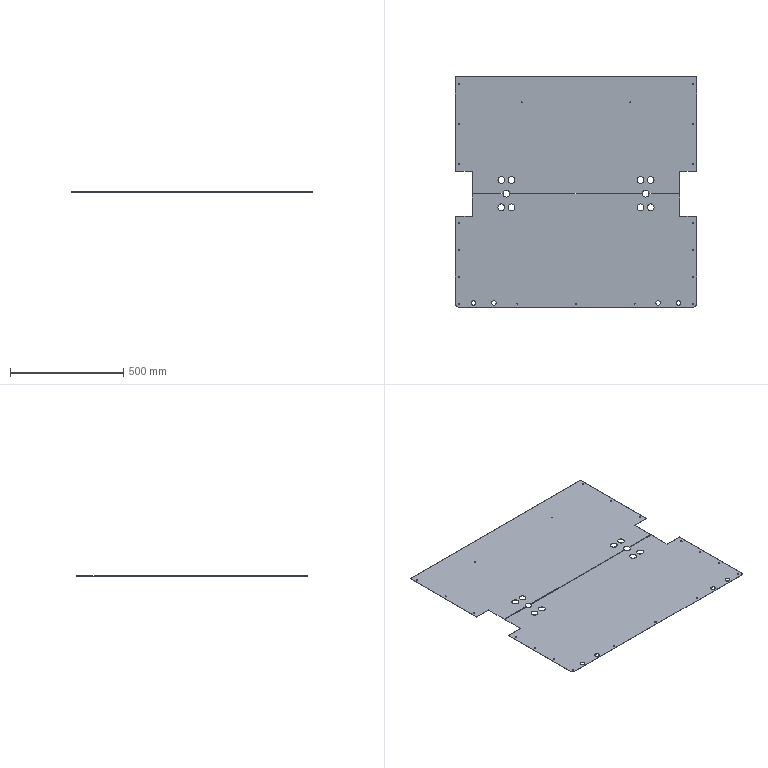Part | 2 solids | 92 faces | box 1064 x 1015 x 1 mm | volume 1039499 mm3 | cylinder 68 | plane 24 | commonest cylinder face diameters 5 x34 30 x20 20 x8 4.5 x4 24 x2